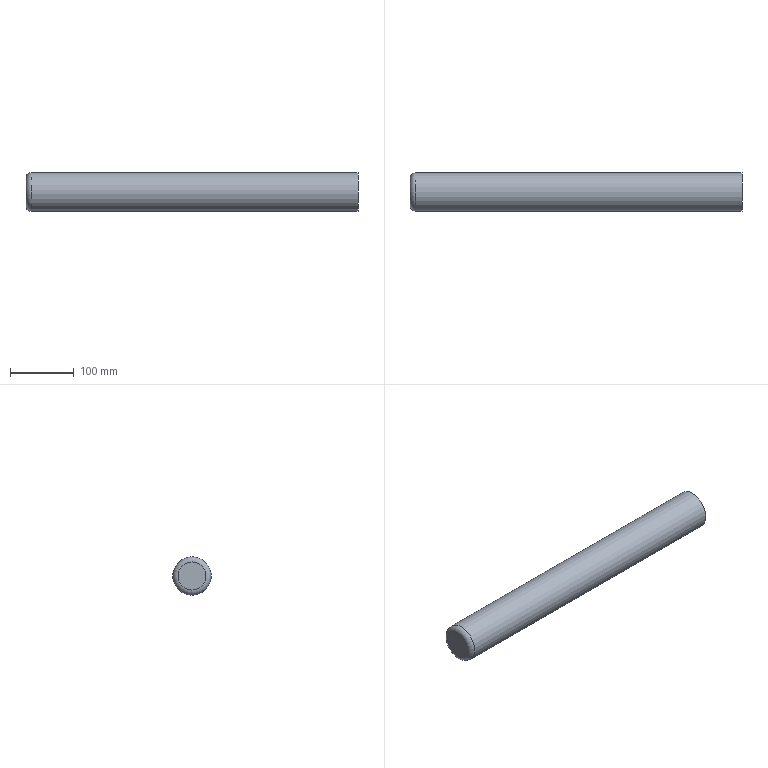Part | STEP file | solid 253 | 1 solid | 4 faces | box 520 x 60 x 60 mm | volume 1467831 mm3 | plane 2 | cylinder 1 | torus 1 | commonest cylinder face diameters 60 x1